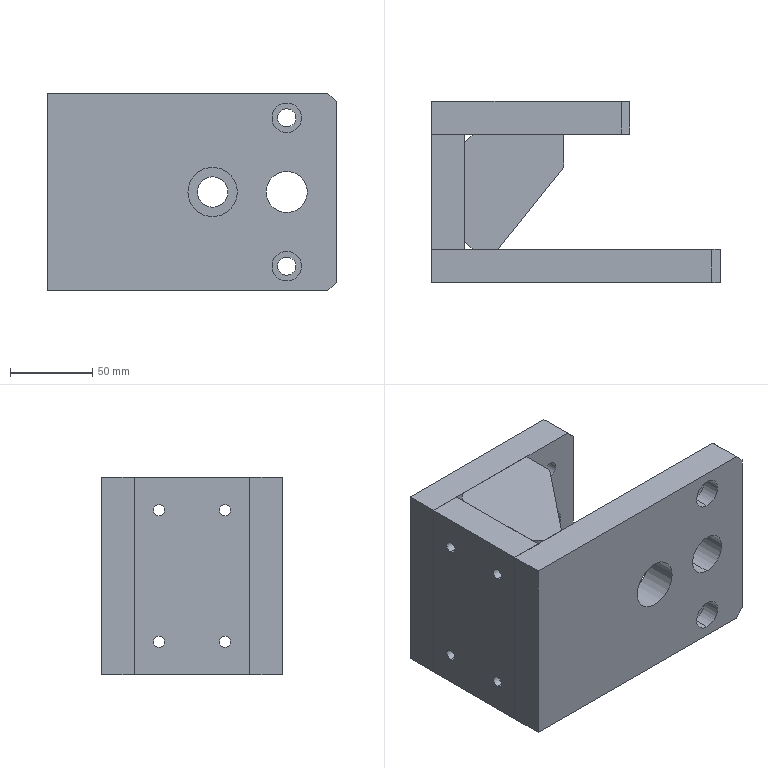Part | SolidWorks | features BaseBody 5 | 5 solids | 68 faces | box 175 x 110 x 120 mm | volume 895687 mm3 | plane 42 | cylinder 26 | commonest cylinder face diameters 6.8 x8 10.2 x4 11 x4 18 x4 18.5 x2 25 x2